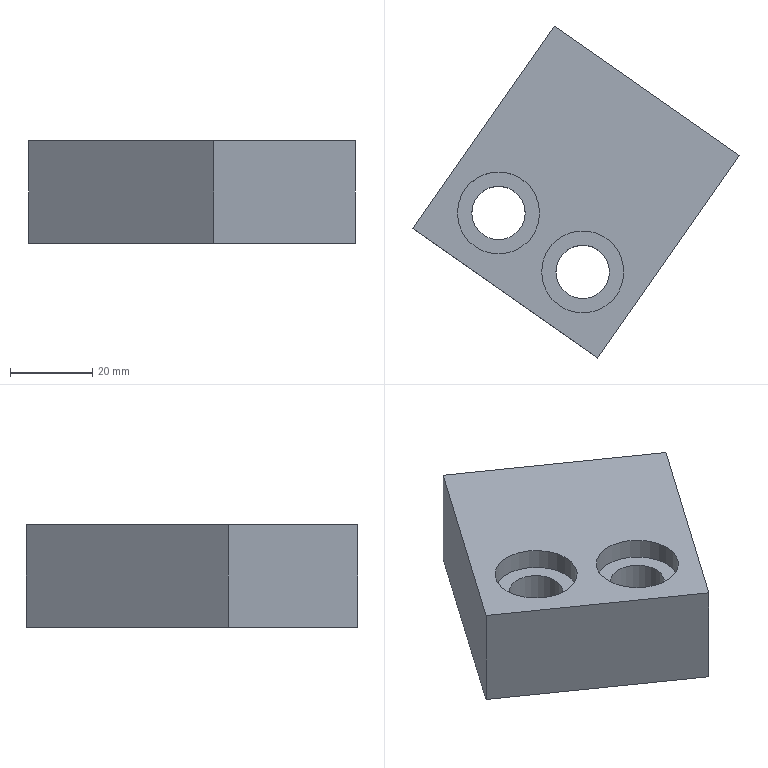Part | NX | features solid 2 | 1 solid | 12 faces | box 79.468 x 80.696 x 25 mm | volume 74049 mm3 | plane 8 | cylinder 4 | commonest cylinder face diameters 13 x2 20 x2
STEP:
#1=CARTESIAN_POINT('',(23.436,-40.826,-125.));
#2=VERTEX_POINT('',#1);
#3=CARTESIAN_POINT('',(-21.617,-9.279,-125.));
#4=VERTEX_POINT('',#3);
#5=CARTESIAN_POINT('',(19.341,-37.958,-125.));
#6=DIRECTION('',(0.8192,-0.5736,0.));
#7=VECTOR('',#6,1000.);
#8=LINE('',#5,#7);
#9=EDGE_CURVE('',#2,#4,#8,.F.);
#10=ORIENTED_EDGE('',*,*,#9,.T.);
#11=CARTESIAN_POINT('',(-21.617,-9.279,-100.));
#12=VERTEX_POINT('',#11);
#13=CARTESIAN_POINT('',(-21.617,-9.279,-100.));
#14=DIRECTION('',(0.,0.,-1.));
#15=VECTOR('',#14,1000.);
#16=LINE('',#13,#15);
#17=EDGE_CURVE('',#12,#4,#16,.T.);
#18=ORIENTED_EDGE('',*,*,#17,.F.);
#19=CARTESIAN_POINT('',(23.436,-40.826,-100.));
#20=VERTEX_POINT('',#19);
#21=CARTESIAN_POINT('',(19.341,-37.958,-100.));
#22=DIRECTION('',(0.8192,-0.5736,0.));
#23=VECTOR('',#22,1000.);
#24=LINE('',#21,#23);
#25=EDGE_CURVE('',#20,#12,#24,.F.);
#26=ORIENTED_EDGE('',*,*,#25,.F.);
#27=CARTESIAN_POINT('',(23.436,-40.826,-100.));
#28=DIRECTION('',(0.,0.,-1.));
#29=VECTOR('',#28,1000.);
#30=LINE('',#27,#29);
#31=EDGE_CURVE('',#20,#2,#30,.T.);
#32=ORIENTED_EDGE('',*,*,#31,.T.);
#33=EDGE_LOOP('',(#10,#18,#26,#32));
#34=FACE_BOUND('',#33,.T.);
#35=CARTESIAN_POINT('',(19.341,-37.958,-100.));
#36=DIRECTION('',(-0.5736,-0.8192,0.));
#37=DIRECTION('',(0.8192,-0.5736,0.));
#38=AXIS2_PLACEMENT_3D('',#35,#36,#37);
#39=PLANE('',#38);
#40=ADVANCED_FACE('',(#34),#39,.F.);
#41=CARTESIAN_POINT('',(-56.031,-58.428,-125.));
#42=VERTEX_POINT('',#41);
#43=CARTESIAN_POINT('',(245.304,371.923,-125.));
#44=DIRECTION('',(0.5736,0.8192,0.));
#45=VECTOR('',#44,1000.);
#46=LINE('',#43,#45);
#47=EDGE_CURVE('',#4,#42,#46,.F.);
#48=ORIENTED_EDGE('',*,*,#47,.T.);
#49=CARTESIAN_POINT('',(-56.031,-58.428,-100.));
#50=VERTEX_POINT('',#49);
#51=CARTESIAN_POINT('',(-56.031,-58.428,-100.));
#52=DIRECTION('',(0.,0.,-1.));
#53=VECTOR('',#52,1000.);
#54=LINE('',#51,#53);
#55=EDGE_CURVE('',#50,#42,#54,.T.);
#56=ORIENTED_EDGE('',*,*,#55,.F.);
#57=CARTESIAN_POINT('',(245.304,371.923,-100.));
#58=DIRECTION('',(0.5736,0.8192,0.));
#59=VECTOR('',#58,1000.);
#60=LINE('',#57,#59);
#61=EDGE_CURVE('',#12,#50,#60,.F.);
#62=ORIENTED_EDGE('',*,*,#61,.F.);
#63=ORIENTED_EDGE('',*,*,#17,.T.);
#64=EDGE_LOOP('',(#48,#56,#62,#63));
#65=FACE_BOUND('',#64,.T.);
#66=CARTESIAN_POINT('',(245.304,371.923,-100.));
#67=DIRECTION('',(0.8192,-0.5736,0.));
#68=DIRECTION('',(0.5736,0.8192,0.));
#69=AXIS2_PLACEMENT_3D('',#66,#67,#68);
#70=PLANE('',#69);
#71=ADVANCED_FACE('',(#65),#70,.F.);
#72=CARTESIAN_POINT('',(-10.978,-89.975,-125.));
#73=VERTEX_POINT('',#72);
#74=CARTESIAN_POINT('',(-19.17,-84.239,-125.));
#75=DIRECTION('',(0.8192,-0.5736,0.));
#76=VECTOR('',#75,1000.);
#77=LINE('',#74,#76);
#78=EDGE_CURVE('',#73,#42,#77,.F.);
#79=ORIENTED_EDGE('',*,*,#78,.F.);
#80=CARTESIAN_POINT('',(-10.978,-89.975,-100.));
#81=VERTEX_POINT('',#80);
#82=CARTESIAN_POINT('',(-10.978,-89.975,-100.));
#83=DIRECTION('',(0.,0.,-1.));
#84=VECTOR('',#83,1000.);
#85=LINE('',#82,#84);
#86=EDGE_CURVE('',#81,#73,#85,.T.);
#87=ORIENTED_EDGE('',*,*,#86,.F.);
#88=CARTESIAN_POINT('',(-19.17,-84.239,-100.));
#89=DIRECTION('',(0.8192,-0.5736,0.));
#90=VECTOR('',#89,1000.);
#91=LINE('',#88,#90);
#92=EDGE_CURVE('',#81,#50,#91,.F.);
#93=ORIENTED_EDGE('',*,*,#92,.T.);
#94=ORIENTED_EDGE('',*,*,#55,.T.);
#95=EDGE_LOOP('',(#79,#87,#93,#94));
#96=FACE_BOUND('',#95,.T.);
#97=CARTESIAN_POINT('',(-19.17,-84.239,-15.));
#98=DIRECTION('',(-0.5736,-0.8192,0.));
#99=DIRECTION('',(0.8192,-0.5736,0.));
#100=AXIS2_PLACEMENT_3D('',#97,#98,#99);
#101=PLANE('',#100);
#102=ADVANCED_FACE('',(#96),#101,.T.);
#103=CARTESIAN_POINT('',(29.172,-32.634,-125.));
#104=DIRECTION('',(0.5736,0.8192,0.));
#105=VECTOR('',#104,1000.);
#106=LINE('',#103,#105);
#107=EDGE_CURVE('',#2,#73,#106,.F.);
#108=ORIENTED_EDGE('',*,*,#107,.F.);
#109=ORIENTED_EDGE('',*,*,#31,.F.);
#110=CARTESIAN_POINT('',(29.172,-32.634,-100.));
#111=DIRECTION('',(0.5736,0.8192,0.));
#112=VECTOR('',#111,1000.);
#113=LINE('',#110,#112);
#114=EDGE_CURVE('',#20,#81,#113,.F.);
#115=ORIENTED_EDGE('',*,*,#114,.T.);
#116=ORIENTED_EDGE('',*,*,#86,.T.);
#117=EDGE_LOOP('',(#108,#109,#115,#116));
#118=FACE_BOUND('',#117,.T.);
#119=CARTESIAN_POINT('',(29.172,-32.634,-100.));
#120=DIRECTION('',(0.8192,-0.5736,0.));
#121=DIRECTION('',(0.5736,0.8192,0.));
#122=AXIS2_PLACEMENT_3D('',#119,#120,#121);
#123=PLANE('',#122);
#124=ADVANCED_FACE('',(#118),#123,.T.);
#125=CARTESIAN_POINT('',(-24.662,-69.084,-100.));
#126=VERTEX_POINT('',#125);
#127=CARTESIAN_POINT('',(-14.662,-69.084,-100.));
#128=DIRECTION('',(0.,0.,-1.));
#129=DIRECTION('',(-1.,0.,0.));
#130=AXIS2_PLACEMENT_3D('',#127,#128,#129);
#131=CIRCLE('',#130,10.);
#132=EDGE_CURVE('',#126,#126,#131,.F.);
#133=ORIENTED_EDGE('',*,*,#132,.F.);
#134=EDGE_LOOP('',(#133));
#135=FACE_BOUND('',#134,.T.);
#136=CARTESIAN_POINT('',(-45.141,-54.745,-100.));
#137=VERTEX_POINT('',#136);
#138=CARTESIAN_POINT('',(-35.141,-54.745,-100.));
#139=DIRECTION('',(0.,0.,-1.));
#140=DIRECTION('',(-1.,0.,0.));
#141=AXIS2_PLACEMENT_3D('',#138,#139,#140);
#142=CIRCLE('',#141,10.);
#143=EDGE_CURVE('',#137,#137,#142,.F.);
#144=ORIENTED_EDGE('',*,*,#143,.F.);
#145=EDGE_LOOP('',(#144));
#146=FACE_BOUND('',#145,.T.);
#147=ORIENTED_EDGE('',*,*,#25,.T.);
#148=ORIENTED_EDGE('',*,*,#61,.T.);
#149=ORIENTED_EDGE('',*,*,#92,.F.);
#150=ORIENTED_EDGE('',*,*,#114,.F.);
#151=EDGE_LOOP('',(#147,#148,#149,#150));
#152=FACE_BOUND('',#151,.T.);
#153=CARTESIAN_POINT('',(780.561,-2.868,-100.));
#154=DIRECTION('',(0.,0.,-1.));
#155=DIRECTION('',(-1.,0.,0.));
#156=AXIS2_PLACEMENT_3D('',#153,#154,#155);
#157=PLANE('',#156);
#158=ADVANCED_FACE('',(#135,#146,#152),#157,.F.);
#159=CARTESIAN_POINT('',(-21.162,-69.084,-125.));
#160=VERTEX_POINT('',#159);
#161=CARTESIAN_POINT('',(-14.662,-69.084,-125.));
#162=DIRECTION('',(0.,0.,-1.));
#163=DIRECTION('',(-1.,0.,0.));
#164=AXIS2_PLACEMENT_3D('',#161,#162,#163);
#165=CIRCLE('',#164,6.5);
#166=EDGE_CURVE('',#160,#160,#165,.F.);
#167=ORIENTED_EDGE('',*,*,#166,.T.);
#168=EDGE_LOOP('',(#167));
#169=FACE_BOUND('',#168,.T.);
#170=CARTESIAN_POINT('',(-41.641,-54.745,-125.));
#171=VERTEX_POINT('',#170);
#172=CARTESIAN_POINT('',(-35.141,-54.745,-125.));
#173=DIRECTION('',(0.,0.,-1.));
#174=DIRECTION('',(-1.,0.,0.));
#175=AXIS2_PLACEMENT_3D('',#172,#173,#174);
#176=CIRCLE('',#175,6.5);
#177=EDGE_CURVE('',#171,#171,#176,.F.);
#178=ORIENTED_EDGE('',*,*,#177,.T.);
#179=EDGE_LOOP('',(#178));
#180=FACE_BOUND('',#179,.T.);
#181=ORIENTED_EDGE('',*,*,#9,.F.);
#182=ORIENTED_EDGE('',*,*,#107,.T.);
#183=ORIENTED_EDGE('',*,*,#78,.T.);
#184=ORIENTED_EDGE('',*,*,#47,.F.);
#185=EDGE_LOOP('',(#181,#182,#183,#184));
#186=FACE_BOUND('',#185,.T.);
#187=CARTESIAN_POINT('',(780.561,-2.868,-125.));
#188=DIRECTION('',(0.,0.,-1.));
#189=DIRECTION('',(-1.,0.,0.));
#190=AXIS2_PLACEMENT_3D('',#187,#188,#189);
#191=PLANE('',#190);
#192=ADVANCED_FACE('',(#169,#180,#186),#191,.T.);
#193=CARTESIAN_POINT('',(-41.641,-54.745,-105.));
#194=VERTEX_POINT('',#193);
#195=CARTESIAN_POINT('',(-35.141,-54.745,-105.));
#196=DIRECTION('',(0.,0.,-1.));
#197=DIRECTION('',(-1.,0.,0.));
#198=AXIS2_PLACEMENT_3D('',#195,#196,#197);
#199=CIRCLE('',#198,6.5);
#200=EDGE_CURVE('',#194,#194,#199,.F.);
#201=ORIENTED_EDGE('',*,*,#200,.T.);
#202=EDGE_LOOP('',(#201));
#203=FACE_BOUND('',#202,.T.);
#204=ORIENTED_EDGE('',*,*,#177,.F.);
#205=EDGE_LOOP('',(#204));
#206=FACE_BOUND('',#205,.T.);
#207=CARTESIAN_POINT('',(-35.141,-54.745,-145.));
#208=DIRECTION('',(0.,0.,1.));
#209=DIRECTION('',(1.,0.,0.));
#210=AXIS2_PLACEMENT_3D('',#207,#208,#209);
#211=CYLINDRICAL_SURFACE('',#210,6.5);
#212=ADVANCED_FACE('',(#203,#206),#211,.F.);
#213=ORIENTED_EDGE('',*,*,#200,.F.);
#214=EDGE_LOOP('',(#213));
#215=FACE_BOUND('',#214,.T.);
#216=CARTESIAN_POINT('',(-25.141,-54.745,-105.));
#217=VERTEX_POINT('',#216);
#218=CARTESIAN_POINT('',(-35.141,-54.745,-105.));
#219=DIRECTION('',(0.,0.,1.));
#220=DIRECTION('',(1.,0.,0.));
#221=AXIS2_PLACEMENT_3D('',#218,#219,#220);
#222=CIRCLE('',#221,10.);
#223=EDGE_CURVE('',#217,#217,#222,.T.);
#224=ORIENTED_EDGE('',*,*,#223,.T.);
#225=EDGE_LOOP('',(#224));
#226=FACE_BOUND('',#225,.T.);
#227=CARTESIAN_POINT('',(-35.141,-54.745,-105.));
#228=DIRECTION('',(0.,0.,-1.));
#229=DIRECTION('',(-1.,0.,0.));
#230=AXIS2_PLACEMENT_3D('',#227,#228,#229);
#231=PLANE('',#230);
#232=ADVANCED_FACE('',(#215,#226),#231,.F.);
#233=ORIENTED_EDGE('',*,*,#143,.T.);
#234=EDGE_LOOP('',(#233));
#235=FACE_BOUND('',#234,.T.);
#236=ORIENTED_EDGE('',*,*,#223,.F.);
#237=EDGE_LOOP('',(#236));
#238=FACE_BOUND('',#237,.T.);
#239=CARTESIAN_POINT('',(-35.141,-54.745,-105.));
#240=DIRECTION('',(0.,0.,1.));
#241=DIRECTION('',(1.,0.,0.));
#242=AXIS2_PLACEMENT_3D('',#239,#240,#241);
#243=CYLINDRICAL_SURFACE('',#242,10.);
#244=ADVANCED_FACE('',(#235,#238),#243,.F.);
#245=CARTESIAN_POINT('',(-21.162,-69.084,-105.));
#246=VERTEX_POINT('',#245);
#247=CARTESIAN_POINT('',(-14.662,-69.084,-105.));
#248=DIRECTION('',(0.,0.,-1.));
#249=DIRECTION('',(-1.,0.,0.));
#250=AXIS2_PLACEMENT_3D('',#247,#248,#249);
#251=CIRCLE('',#250,6.5);
#252=EDGE_CURVE('',#246,#246,#251,.F.);
#253=ORIENTED_EDGE('',*,*,#252,.T.);
#254=EDGE_LOOP('',(#253));
#255=FACE_BOUND('',#254,.T.);
#256=ORIENTED_EDGE('',*,*,#166,.F.);
#257=EDGE_LOOP('',(#256));
#258=FACE_BOUND('',#257,.T.);
#259=CARTESIAN_POINT('',(-14.662,-69.084,-145.));
#260=DIRECTION('',(0.,0.,1.));
#261=DIRECTION('',(1.,0.,0.));
#262=AXIS2_PLACEMENT_3D('',#259,#260,#261);
#263=CYLINDRICAL_SURFACE('',#262,6.5);
#264=ADVANCED_FACE('',(#255,#258),#263,.F.);
#265=ORIENTED_EDGE('',*,*,#252,.F.);
#266=EDGE_LOOP('',(#265));
#267=FACE_BOUND('',#266,.T.);
#268=CARTESIAN_POINT('',(-4.662,-69.084,-105.));
#269=VERTEX_POINT('',#268);
#270=CARTESIAN_POINT('',(-14.662,-69.084,-105.));
#271=DIRECTION('',(0.,0.,1.));
#272=DIRECTION('',(1.,0.,0.));
#273=AXIS2_PLACEMENT_3D('',#270,#271,#272);
#274=CIRCLE('',#273,10.);
#275=EDGE_CURVE('',#269,#269,#274,.T.);
#276=ORIENTED_EDGE('',*,*,#275,.T.);
#277=EDGE_LOOP('',(#276));
#278=FACE_BOUND('',#277,.T.);
#279=CARTESIAN_POINT('',(-14.662,-69.084,-105.));
#280=DIRECTION('',(0.,0.,-1.));
#281=DIRECTION('',(-1.,0.,0.));
#282=AXIS2_PLACEMENT_3D('',#279,#280,#281);
#283=PLANE('',#282);
#284=ADVANCED_FACE('',(#267,#278),#283,.F.);
#285=ORIENTED_EDGE('',*,*,#132,.T.);
#286=EDGE_LOOP('',(#285));
#287=FACE_BOUND('',#286,.T.);
#288=ORIENTED_EDGE('',*,*,#275,.F.);
#289=EDGE_LOOP('',(#288));
#290=FACE_BOUND('',#289,.T.);
#291=CARTESIAN_POINT('',(-14.662,-69.084,-105.));
#292=DIRECTION('',(0.,0.,1.));
#293=DIRECTION('',(1.,0.,0.));
#294=AXIS2_PLACEMENT_3D('',#291,#292,#293);
#295=CYLINDRICAL_SURFACE('',#294,10.);
#296=ADVANCED_FACE('',(#287,#290),#295,.F.);
#297=CLOSED_SHELL('',(#40,#71,#102,#124,#158,#192,#212,#232,#244,#264,#284,#296));
#298=MANIFOLD_SOLID_BREP('',#297);
#299=(LENGTH_UNIT()NAMED_UNIT(*)SI_UNIT(.MILLI.,.METRE.));
#300=UNCERTAINTY_MEASURE_WITH_UNIT(LENGTH_MEASURE(0.00001),#299,'','');
#301=(NAMED_UNIT(*)PLANE_ANGLE_UNIT()SI_UNIT($,.RADIAN.));
#302=(NAMED_UNIT(*)SI_UNIT($,.STERADIAN.)SOLID_ANGLE_UNIT());
#303=(GEOMETRIC_REPRESENTATION_CONTEXT(3)GLOBAL_UNCERTAINTY_ASSIGNED_CONTEXT((#300))GLOBAL_UNIT_ASSIGNED_CONTEXT((#299,#301,#302))REPRESENTATION_CONTEXT('',''));
#304=ADVANCED_BREP_SHAPE_REPRESENTATION('',(#298),#303);